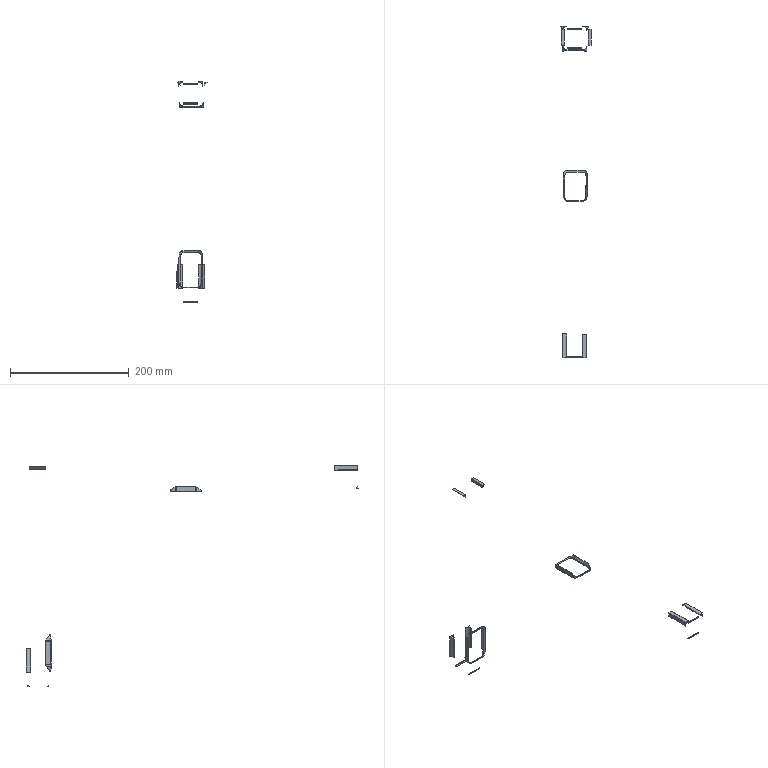Part | STEP file | R1_01_rama_Spoiny | 12 solids | 132 faces | box 50.98 x 559.497 x 372.642 mm | volume 5856 mm3 | plane 84 | spline 40 | cylinder 8 | commonest cylinder face diameters 13.2 x8